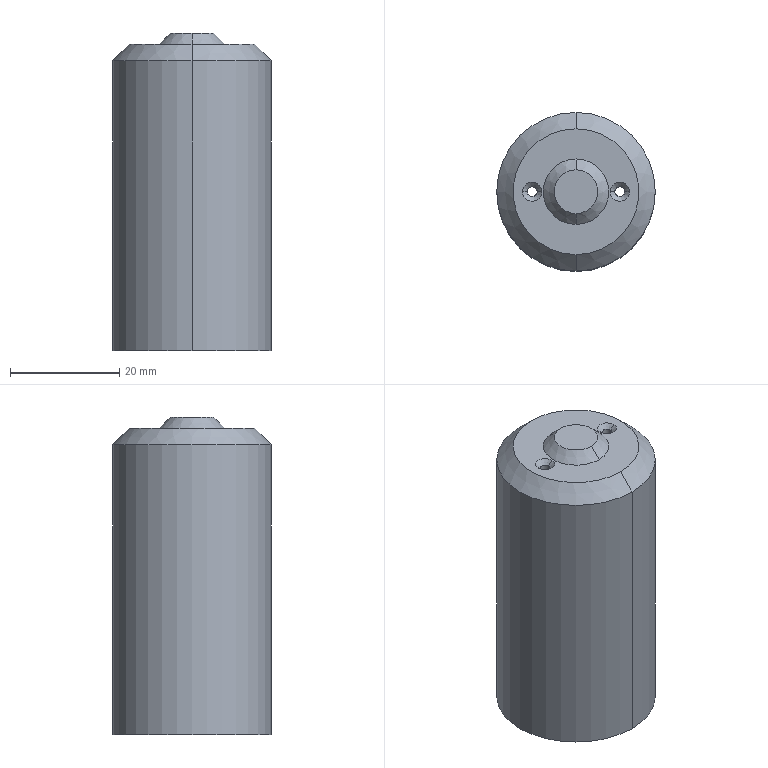Part | STEP file | ASND-0110-4216225600 | 1 solid | 25 faces | box 29 x 29 x 58 mm | volume 3832 mm3 | cone 12 | cylinder 8 | plane 5 | commonest cylinder face diameters 1.8 x4 28 x2 29 x2